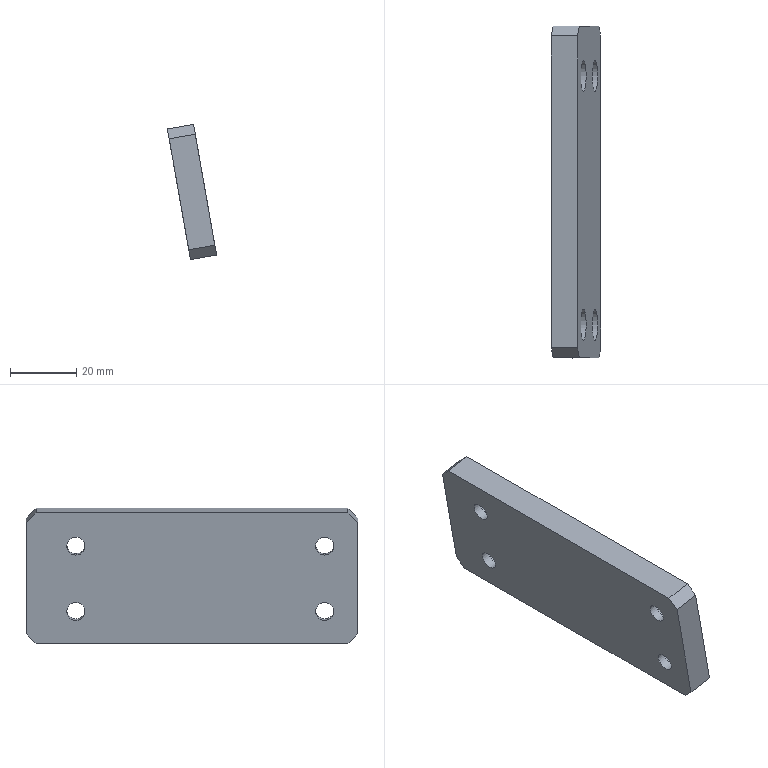Part | STEP file | P011002S002-007 | 1 solid | 22 faces | box 14.824 x 100 x 40.781 mm | volume 30059 mm3 | plane 14 | cylinder 8 | commonest cylinder face diameters 5.5 x4 9.5 x4